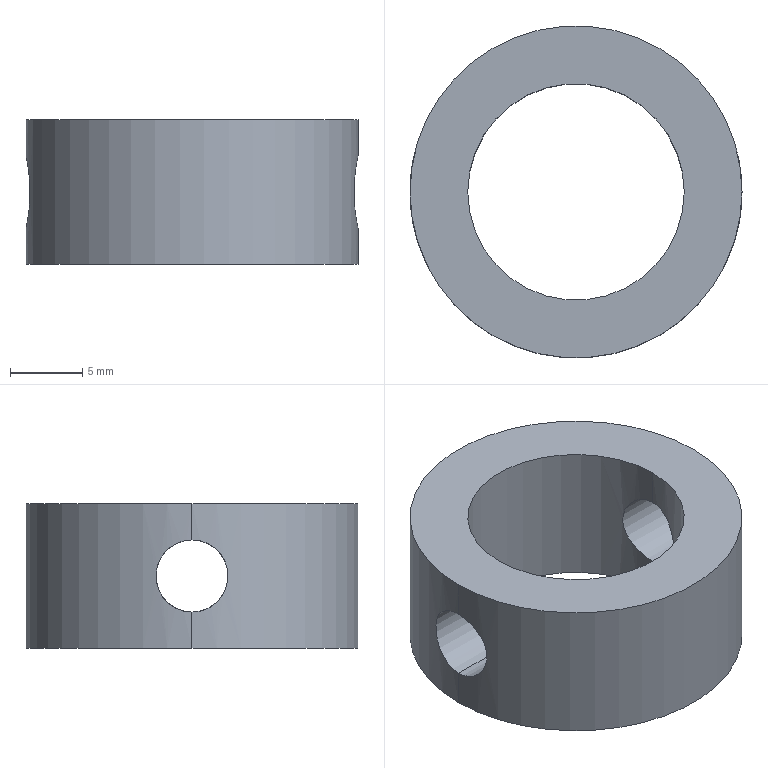Part | STEP file | X77b-01013 | 1 solid | 10 faces | box 23 x 23 x 10 mm | volume 2229 mm3 | cylinder 8 | plane 2 | commonest cylinder face diameters 5 x4 15 x2 23 x2
STEP:
#1=CARTESIAN_POINT('',(-11.5,0.,7.5));
#2=VERTEX_POINT('',#1);
#3=CARTESIAN_POINT('',(-11.5,0.,2.5));
#4=VERTEX_POINT('',#3);
#5=CARTESIAN_POINT('',(-11.5,0.,7.5));
#6=CARTESIAN_POINT('',(-11.5,-0.3268,7.5));
#7=CARTESIAN_POINT('',(-11.485,-0.6567,7.434));
#8=CARTESIAN_POINT('',(-11.447,-1.108,7.247));
#9=CARTESIAN_POINT('',(-11.432,-1.254,7.169));
#10=CARTESIAN_POINT('',(-11.399,-1.526,6.987));
#11=CARTESIAN_POINT('',(-11.381,-1.652,6.884));
#12=CARTESIAN_POINT('',(-11.346,-1.882,6.654));
#13=CARTESIAN_POINT('',(-11.327,-1.987,6.525));
#14=CARTESIAN_POINT('',(-11.294,-2.168,6.255));
#15=CARTESIAN_POINT('',(-11.279,-2.245,6.112));
#16=CARTESIAN_POINT('',(-11.24,-2.435,5.656));
#17=CARTESIAN_POINT('',(-11.225,-2.5,5.331));
#18=CARTESIAN_POINT('',(-11.225,-2.5,4.836));
#19=CARTESIAN_POINT('',(-11.229,-2.484,4.673));
#20=CARTESIAN_POINT('',(-11.242,-2.42,4.353));
#21=CARTESIAN_POINT('',(-11.253,-2.372,4.193));
#22=CARTESIAN_POINT('',(-11.279,-2.247,3.892));
#23=CARTESIAN_POINT('',(-11.294,-2.17,3.748));
#24=CARTESIAN_POINT('',(-11.327,-1.988,3.476));
#25=CARTESIAN_POINT('',(-11.345,-1.884,3.348));
#26=CARTESIAN_POINT('',(-11.399,-1.539,3.004));
#27=CARTESIAN_POINT('',(-11.435,-1.261,2.817));
#28=CARTESIAN_POINT('',(-11.472,-0.8104,2.629));
#29=CARTESIAN_POINT('',(-11.483,-0.6516,2.581));
#30=CARTESIAN_POINT('',(-11.496,-0.3291,2.516));
#31=CARTESIAN_POINT('',(-11.5,-0.1657,2.5));
#32=CARTESIAN_POINT('',(-11.5,0.,2.5));
#33=B_SPLINE_CURVE_WITH_KNOTS('',3,(#5,#6,#7,#8,#9,#10,#11,#12,#13,#14,#15,#16,#17,#18,#19,#20,#21,#22,#23,#24,#25,#26,#27,#28,#29,#30,#31,#32),.UNSPECIFIED.,.F.,.F.,(4,2,2,2,2,2,2,2,2,2,2,2,2,4),(0.00784,0.008819,0.009309,0.009799,0.01029,0.01078,0.01176,0.01225,0.01274,0.01323,0.01372,0.0147,0.01519,0.01568),.UNSPECIFIED.);
#34=EDGE_CURVE('',#2,#4,#33,.T.);
#35=ORIENTED_EDGE('',*,*,#34,.F.);
#36=CARTESIAN_POINT('',(-7.5,0.,7.5));
#37=VERTEX_POINT('',#36);
#38=CARTESIAN_POINT('',(-11.5,0.,7.5));
#39=DIRECTION('',(1.,0.,0.));
#40=VECTOR('',#39,1000.);
#41=LINE('',#38,#40);
#42=EDGE_CURVE('',#2,#37,#41,.T.);
#43=ORIENTED_EDGE('',*,*,#42,.T.);
#44=CARTESIAN_POINT('',(-7.5,0.,2.5));
#45=VERTEX_POINT('',#44);
#46=CARTESIAN_POINT('',(-7.5,0.,7.5));
#47=CARTESIAN_POINT('',(-7.5,-0.1665,7.5));
#48=CARTESIAN_POINT('',(-7.494,-0.3299,7.484));
#49=CARTESIAN_POINT('',(-7.473,-0.6511,7.419));
#50=CARTESIAN_POINT('',(-7.458,-0.8106,7.371));
#51=CARTESIAN_POINT('',(-7.419,-1.113,7.245));
#52=CARTESIAN_POINT('',(-7.395,-1.256,7.168));
#53=CARTESIAN_POINT('',(-7.344,-1.527,6.986));
#54=CARTESIAN_POINT('',(-7.316,-1.654,6.881));
#55=CARTESIAN_POINT('',(-7.233,-1.997,6.538));
#56=CARTESIAN_POINT('',(-7.176,-2.183,6.261));
#57=CARTESIAN_POINT('',(-7.116,-2.37,5.811));
#58=CARTESIAN_POINT('',(-7.099,-2.419,5.652));
#59=CARTESIAN_POINT('',(-7.077,-2.484,5.329));
#60=CARTESIAN_POINT('',(-7.071,-2.5,5.166));
#61=CARTESIAN_POINT('',(-7.071,-2.5,4.837));
#62=CARTESIAN_POINT('',(-7.077,-2.484,4.67));
#63=CARTESIAN_POINT('',(-7.099,-2.419,4.348));
#64=CARTESIAN_POINT('',(-7.116,-2.371,4.192));
#65=CARTESIAN_POINT('',(-7.156,-2.245,3.887));
#66=CARTESIAN_POINT('',(-7.181,-2.167,3.743));
#67=CARTESIAN_POINT('',(-7.233,-1.987,3.474));
#68=CARTESIAN_POINT('',(-7.261,-1.882,3.347));
#69=CARTESIAN_POINT('',(-7.317,-1.652,3.117));
#70=CARTESIAN_POINT('',(-7.344,-1.527,3.014));
#71=CARTESIAN_POINT('',(-7.395,-1.257,2.833));
#72=CARTESIAN_POINT('',(-7.419,-1.111,2.754));
#73=CARTESIAN_POINT('',(-7.458,-0.8095,2.629));
#74=CARTESIAN_POINT('',(-7.473,-0.6534,2.581));
#75=CARTESIAN_POINT('',(-7.495,-0.3297,2.516));
#76=CARTESIAN_POINT('',(-7.5,-0.164,2.5));
#77=CARTESIAN_POINT('',(-7.5,0.,2.5));
#78=B_SPLINE_CURVE_WITH_KNOTS('',3,(#46,#47,#48,#49,#50,#51,#52,#53,#54,#55,#56,#57,#58,#59,#60,#61,#62,#63,#64,#65,#66,#67,#68,#69,#70,#71,#72,#73,#74,#75,#76,#77),.UNSPECIFIED.,.F.,.F.,(4,2,2,2,2,2,2,2,2,2,2,2,2,2,2,4),(0.,0.0004921,0.0009841,0.001476,0.001968,0.002952,0.003444,0.003936,0.004429,0.004921,0.005413,0.005905,0.006397,0.006889,0.007381,0.007873),.UNSPECIFIED.);
#79=EDGE_CURVE('',#37,#45,#78,.T.);
#80=ORIENTED_EDGE('',*,*,#79,.T.);
#81=CARTESIAN_POINT('',(-11.5,0.,2.5));
#82=DIRECTION('',(1.,0.,0.));
#83=VECTOR('',#82,1000.);
#84=LINE('',#81,#83);
#85=EDGE_CURVE('',#4,#45,#84,.T.);
#86=ORIENTED_EDGE('',*,*,#85,.F.);
#87=EDGE_LOOP('',(#35,#43,#80,#86));
#88=FACE_OUTER_BOUND('',#87,.T.);
#89=CARTESIAN_POINT('',(-11.5,0.,5.));
#90=DIRECTION('',(1.,0.,0.));
#91=DIRECTION('',(0.,0.,-1.));
#92=AXIS2_PLACEMENT_3D('',#89,#90,#91);
#93=CYLINDRICAL_SURFACE('',#92,2.5);
#94=ADVANCED_FACE('',(#88),#93,.F.);
#95=CARTESIAN_POINT('',(7.5,0.,2.5));
#96=VERTEX_POINT('',#95);
#97=CARTESIAN_POINT('',(7.5,0.,7.5));
#98=VERTEX_POINT('',#97);
#99=CARTESIAN_POINT('',(7.5,0.,2.5));
#100=CARTESIAN_POINT('',(7.5,-0.1665,2.5));
#101=CARTESIAN_POINT('',(7.494,-0.3299,2.516));
#102=CARTESIAN_POINT('',(7.473,-0.6511,2.581));
#103=CARTESIAN_POINT('',(7.458,-0.8106,2.629));
#104=CARTESIAN_POINT('',(7.419,-1.113,2.755));
#105=CARTESIAN_POINT('',(7.395,-1.256,2.832));
#106=CARTESIAN_POINT('',(7.344,-1.527,3.014));
#107=CARTESIAN_POINT('',(7.316,-1.654,3.119));
#108=CARTESIAN_POINT('',(7.233,-1.997,3.462));
#109=CARTESIAN_POINT('',(7.176,-2.183,3.739));
#110=CARTESIAN_POINT('',(7.116,-2.37,4.189));
#111=CARTESIAN_POINT('',(7.099,-2.419,4.348));
#112=CARTESIAN_POINT('',(7.077,-2.484,4.671));
#113=CARTESIAN_POINT('',(7.071,-2.5,4.834));
#114=CARTESIAN_POINT('',(7.071,-2.5,5.163));
#115=CARTESIAN_POINT('',(7.077,-2.484,5.33));
#116=CARTESIAN_POINT('',(7.099,-2.419,5.652));
#117=CARTESIAN_POINT('',(7.116,-2.371,5.808));
#118=CARTESIAN_POINT('',(7.156,-2.245,6.113));
#119=CARTESIAN_POINT('',(7.181,-2.167,6.257));
#120=CARTESIAN_POINT('',(7.233,-1.987,6.526));
#121=CARTESIAN_POINT('',(7.261,-1.882,6.653));
#122=CARTESIAN_POINT('',(7.317,-1.652,6.883));
#123=CARTESIAN_POINT('',(7.344,-1.527,6.986));
#124=CARTESIAN_POINT('',(7.395,-1.257,7.167));
#125=CARTESIAN_POINT('',(7.419,-1.111,7.246));
#126=CARTESIAN_POINT('',(7.458,-0.8095,7.371));
#127=CARTESIAN_POINT('',(7.473,-0.6534,7.419));
#128=CARTESIAN_POINT('',(7.495,-0.3297,7.484));
#129=CARTESIAN_POINT('',(7.5,-0.164,7.5));
#130=CARTESIAN_POINT('',(7.5,0.,7.5));
#131=B_SPLINE_CURVE_WITH_KNOTS('',3,(#99,#100,#101,#102,#103,#104,#105,#106,#107,#108,#109,#110,#111,#112,#113,#114,#115,#116,#117,#118,#119,#120,#121,#122,#123,#124,#125,#126,#127,#128,#129,#130),.UNSPECIFIED.,.F.,.F.,(4,2,2,2,2,2,2,2,2,2,2,2,2,2,2,4),(0.,0.0004921,0.0009841,0.001476,0.001968,0.002952,0.003444,0.003936,0.004429,0.004921,0.005413,0.005905,0.006397,0.006889,0.007381,0.007873),.UNSPECIFIED.);
#132=EDGE_CURVE('',#96,#98,#131,.T.);
#133=ORIENTED_EDGE('',*,*,#132,.T.);
#134=CARTESIAN_POINT('',(11.5,0.,7.5));
#135=VERTEX_POINT('',#134);
#136=CARTESIAN_POINT('',(-11.5,0.,7.5));
#137=DIRECTION('',(1.,0.,0.));
#138=VECTOR('',#137,1000.);
#139=LINE('',#136,#138);
#140=EDGE_CURVE('',#98,#135,#139,.T.);
#141=ORIENTED_EDGE('',*,*,#140,.T.);
#142=CARTESIAN_POINT('',(11.5,0.,2.5));
#143=VERTEX_POINT('',#142);
#144=CARTESIAN_POINT('',(11.5,0.,2.5));
#145=CARTESIAN_POINT('',(11.5,-0.1657,2.5));
#146=CARTESIAN_POINT('',(11.496,-0.3286,2.516));
#147=CARTESIAN_POINT('',(11.483,-0.6488,2.58));
#148=CARTESIAN_POINT('',(11.473,-0.8079,2.628));
#149=CARTESIAN_POINT('',(11.447,-1.11,2.754));
#150=CARTESIAN_POINT('',(11.432,-1.254,2.831));
#151=CARTESIAN_POINT('',(11.399,-1.525,3.012));
#152=CARTESIAN_POINT('',(11.381,-1.653,3.118));
#153=CARTESIAN_POINT('',(11.327,-1.998,3.463));
#154=CARTESIAN_POINT('',(11.291,-2.184,3.741));
#155=CARTESIAN_POINT('',(11.253,-2.371,4.192));
#156=CARTESIAN_POINT('',(11.243,-2.42,4.35));
#157=CARTESIAN_POINT('',(11.229,-2.484,4.673));
#158=CARTESIAN_POINT('',(11.225,-2.5,4.835));
#159=CARTESIAN_POINT('',(11.225,-2.5,5.163));
#160=CARTESIAN_POINT('',(11.229,-2.484,5.329));
#161=CARTESIAN_POINT('',(11.243,-2.42,5.65));
#162=CARTESIAN_POINT('',(11.253,-2.372,5.806));
#163=CARTESIAN_POINT('',(11.279,-2.246,6.109));
#164=CARTESIAN_POINT('',(11.294,-2.168,6.255));
#165=CARTESIAN_POINT('',(11.327,-1.988,6.525));
#166=CARTESIAN_POINT('',(11.345,-1.884,6.652));
#167=CARTESIAN_POINT('',(11.381,-1.651,6.884));
#168=CARTESIAN_POINT('',(11.399,-1.526,6.987));
#169=CARTESIAN_POINT('',(11.432,-1.255,7.168));
#170=CARTESIAN_POINT('',(11.447,-1.109,7.247));
#171=CARTESIAN_POINT('',(11.473,-0.8068,7.372));
#172=CARTESIAN_POINT('',(11.483,-0.651,7.419));
#173=CARTESIAN_POINT('',(11.496,-0.3294,7.484));
#174=CARTESIAN_POINT('',(11.5,-0.1634,7.5));
#175=CARTESIAN_POINT('',(11.5,0.,7.5));
#176=B_SPLINE_CURVE_WITH_KNOTS('',3,(#144,#145,#146,#147,#148,#149,#150,#151,#152,#153,#154,#155,#156,#157,#158,#159,#160,#161,#162,#163,#164,#165,#166,#167,#168,#169,#170,#171,#172,#173,#174,#175),.UNSPECIFIED.,.F.,.F.,(4,2,2,2,2,2,2,2,2,2,2,2,2,2,2,4),(0.,0.00049,0.0009799,0.00147,0.00196,0.00294,0.00343,0.00392,0.00441,0.0049,0.00539,0.00588,0.00637,0.00686,0.00735,0.00784),.UNSPECIFIED.);
#177=EDGE_CURVE('',#143,#135,#176,.T.);
#178=ORIENTED_EDGE('',*,*,#177,.F.);
#179=CARTESIAN_POINT('',(-11.5,0.,2.5));
#180=DIRECTION('',(1.,0.,0.));
#181=VECTOR('',#180,1000.);
#182=LINE('',#179,#181);
#183=EDGE_CURVE('',#96,#143,#182,.T.);
#184=ORIENTED_EDGE('',*,*,#183,.F.);
#185=EDGE_LOOP('',(#133,#141,#178,#184));
#186=FACE_OUTER_BOUND('',#185,.T.);
#187=CARTESIAN_POINT('',(-11.5,0.,5.));
#188=DIRECTION('',(1.,0.,0.));
#189=DIRECTION('',(0.,0.,-1.));
#190=AXIS2_PLACEMENT_3D('',#187,#188,#189);
#191=CYLINDRICAL_SURFACE('',#190,2.5);
#192=ADVANCED_FACE('',(#186),#191,.F.);
#193=CARTESIAN_POINT('',(-7.5,0.,10.));
#194=VERTEX_POINT('',#193);
#195=CARTESIAN_POINT('',(7.5,0.,10.));
#196=VERTEX_POINT('',#195);
#197=CARTESIAN_POINT('',(0.,0.,10.));
#198=DIRECTION('',(0.,0.,1.));
#199=DIRECTION('',(1.,0.,0.));
#200=AXIS2_PLACEMENT_3D('',#197,#198,#199);
#201=CIRCLE('',#200,7.5);
#202=EDGE_CURVE('',#194,#196,#201,.T.);
#203=ORIENTED_EDGE('',*,*,#202,.T.);
#204=CARTESIAN_POINT('',(7.5,0.,10.));
#205=DIRECTION('',(0.,0.,-1.));
#206=VECTOR('',#205,1000.);
#207=LINE('',#204,#206);
#208=EDGE_CURVE('',#196,#98,#207,.T.);
#209=ORIENTED_EDGE('',*,*,#208,.T.);
#210=ORIENTED_EDGE('',*,*,#132,.F.);
#211=CARTESIAN_POINT('',(7.5,0.,0.));
#212=VERTEX_POINT('',#211);
#213=CARTESIAN_POINT('',(7.5,0.,10.));
#214=DIRECTION('',(0.,0.,-1.));
#215=VECTOR('',#214,1000.);
#216=LINE('',#213,#215);
#217=EDGE_CURVE('',#96,#212,#216,.T.);
#218=ORIENTED_EDGE('',*,*,#217,.T.);
#219=CARTESIAN_POINT('',(-7.5,0.,0.));
#220=VERTEX_POINT('',#219);
#221=CARTESIAN_POINT('',(0.,0.,0.));
#222=DIRECTION('',(0.,0.,1.));
#223=DIRECTION('',(1.,0.,0.));
#224=AXIS2_PLACEMENT_3D('',#221,#222,#223);
#225=CIRCLE('',#224,7.5);
#226=EDGE_CURVE('',#220,#212,#225,.T.);
#227=ORIENTED_EDGE('',*,*,#226,.F.);
#228=CARTESIAN_POINT('',(-7.5,0.,10.));
#229=DIRECTION('',(0.,0.,-1.));
#230=VECTOR('',#229,1000.);
#231=LINE('',#228,#230);
#232=EDGE_CURVE('',#45,#220,#231,.T.);
#233=ORIENTED_EDGE('',*,*,#232,.F.);
#234=ORIENTED_EDGE('',*,*,#79,.F.);
#235=CARTESIAN_POINT('',(-7.5,0.,10.));
#236=DIRECTION('',(0.,0.,-1.));
#237=VECTOR('',#236,1000.);
#238=LINE('',#235,#237);
#239=EDGE_CURVE('',#194,#37,#238,.T.);
#240=ORIENTED_EDGE('',*,*,#239,.F.);
#241=EDGE_LOOP('',(#203,#209,#210,#218,#227,#233,#234,#240));
#242=FACE_OUTER_BOUND('',#241,.T.);
#243=CARTESIAN_POINT('',(0.,0.,10.));
#244=DIRECTION('',(0.,0.,-1.));
#245=DIRECTION('',(-1.,0.,0.));
#246=AXIS2_PLACEMENT_3D('',#243,#244,#245);
#247=CYLINDRICAL_SURFACE('',#246,7.5);
#248=ADVANCED_FACE('',(#242),#247,.F.);
#249=CARTESIAN_POINT('',(11.5,0.,10.));
#250=VERTEX_POINT('',#249);
#251=CARTESIAN_POINT('',(-11.5,0.,10.));
#252=VERTEX_POINT('',#251);
#253=CARTESIAN_POINT('',(0.,0.,10.));
#254=DIRECTION('',(0.,0.,1.));
#255=DIRECTION('',(1.,0.,0.));
#256=AXIS2_PLACEMENT_3D('',#253,#254,#255);
#257=CIRCLE('',#256,11.5);
#258=EDGE_CURVE('',#250,#252,#257,.T.);
#259=ORIENTED_EDGE('',*,*,#258,.F.);
#260=CARTESIAN_POINT('',(11.5,0.,10.));
#261=DIRECTION('',(0.,0.,-1.));
#262=VECTOR('',#261,1000.);
#263=LINE('',#260,#262);
#264=EDGE_CURVE('',#250,#135,#263,.T.);
#265=ORIENTED_EDGE('',*,*,#264,.T.);
#266=CARTESIAN_POINT('',(11.5,0.,7.5));
#267=CARTESIAN_POINT('',(11.5,0.3268,7.5));
#268=CARTESIAN_POINT('',(11.485,0.6567,7.434));
#269=CARTESIAN_POINT('',(11.447,1.108,7.247));
#270=CARTESIAN_POINT('',(11.432,1.254,7.169));
#271=CARTESIAN_POINT('',(11.399,1.526,6.987));
#272=CARTESIAN_POINT('',(11.381,1.652,6.884));
#273=CARTESIAN_POINT('',(11.346,1.882,6.654));
#274=CARTESIAN_POINT('',(11.327,1.987,6.525));
#275=CARTESIAN_POINT('',(11.294,2.168,6.255));
#276=CARTESIAN_POINT('',(11.279,2.245,6.112));
#277=CARTESIAN_POINT('',(11.24,2.435,5.656));
#278=CARTESIAN_POINT('',(11.225,2.5,5.331));
#279=CARTESIAN_POINT('',(11.225,2.5,4.836));
#280=CARTESIAN_POINT('',(11.229,2.484,4.673));
#281=CARTESIAN_POINT('',(11.242,2.42,4.353));
#282=CARTESIAN_POINT('',(11.253,2.372,4.193));
#283=CARTESIAN_POINT('',(11.279,2.247,3.892));
#284=CARTESIAN_POINT('',(11.294,2.17,3.748));
#285=CARTESIAN_POINT('',(11.327,1.988,3.476));
#286=CARTESIAN_POINT('',(11.345,1.884,3.348));
#287=CARTESIAN_POINT('',(11.399,1.539,3.004));
#288=CARTESIAN_POINT('',(11.435,1.261,2.817));
#289=CARTESIAN_POINT('',(11.472,0.8104,2.629));
#290=CARTESIAN_POINT('',(11.483,0.6516,2.581));
#291=CARTESIAN_POINT('',(11.496,0.3291,2.516));
#292=CARTESIAN_POINT('',(11.5,0.1657,2.5));
#293=CARTESIAN_POINT('',(11.5,0.,2.5));
#294=B_SPLINE_CURVE_WITH_KNOTS('',3,(#266,#267,#268,#269,#270,#271,#272,#273,#274,#275,#276,#277,#278,#279,#280,#281,#282,#283,#284,#285,#286,#287,#288,#289,#290,#291,#292,#293),.UNSPECIFIED.,.F.,.F.,(4,2,2,2,2,2,2,2,2,2,2,2,2,4),(0.00784,0.008819,0.009309,0.009799,0.01029,0.01078,0.01176,0.01225,0.01274,0.01323,0.01372,0.0147,0.01519,0.01568),.UNSPECIFIED.);
#295=EDGE_CURVE('',#135,#143,#294,.T.);
#296=ORIENTED_EDGE('',*,*,#295,.T.);
#297=CARTESIAN_POINT('',(11.5,0.,0.));
#298=VERTEX_POINT('',#297);
#299=CARTESIAN_POINT('',(11.5,0.,10.));
#300=DIRECTION('',(0.,0.,-1.));
#301=VECTOR('',#300,1000.);
#302=LINE('',#299,#301);
#303=EDGE_CURVE('',#143,#298,#302,.T.);
#304=ORIENTED_EDGE('',*,*,#303,.T.);
#305=CARTESIAN_POINT('',(-11.5,0.,0.));
#306=VERTEX_POINT('',#305);
#307=CARTESIAN_POINT('',(0.,0.,0.));
#308=DIRECTION('',(0.,0.,1.));
#309=DIRECTION('',(1.,0.,0.));
#310=AXIS2_PLACEMENT_3D('',#307,#308,#309);
#311=CIRCLE('',#310,11.5);
#312=EDGE_CURVE('',#298,#306,#311,.T.);
#313=ORIENTED_EDGE('',*,*,#312,.T.);
#314=CARTESIAN_POINT('',(-11.5,0.,10.));
#315=DIRECTION('',(0.,0.,-1.));
#316=VECTOR('',#315,1000.);
#317=LINE('',#314,#316);
#318=EDGE_CURVE('',#4,#306,#317,.T.);
#319=ORIENTED_EDGE('',*,*,#318,.F.);
#320=CARTESIAN_POINT('',(-11.5,0.,2.5));
#321=CARTESIAN_POINT('',(-11.5,0.1657,2.5));
#322=CARTESIAN_POINT('',(-11.496,0.3286,2.516));
#323=CARTESIAN_POINT('',(-11.483,0.6488,2.58));
#324=CARTESIAN_POINT('',(-11.473,0.8079,2.628));
#325=CARTESIAN_POINT('',(-11.447,1.11,2.754));
#326=CARTESIAN_POINT('',(-11.432,1.254,2.831));
#327=CARTESIAN_POINT('',(-11.399,1.525,3.012));
#328=CARTESIAN_POINT('',(-11.381,1.653,3.118));
#329=CARTESIAN_POINT('',(-11.327,1.998,3.463));
#330=CARTESIAN_POINT('',(-11.291,2.184,3.741));
#331=CARTESIAN_POINT('',(-11.253,2.371,4.192));
#332=CARTESIAN_POINT('',(-11.243,2.42,4.35));
#333=CARTESIAN_POINT('',(-11.229,2.484,4.673));
#334=CARTESIAN_POINT('',(-11.225,2.5,4.835));
#335=CARTESIAN_POINT('',(-11.225,2.5,5.163));
#336=CARTESIAN_POINT('',(-11.229,2.484,5.329));
#337=CARTESIAN_POINT('',(-11.243,2.42,5.65));
#338=CARTESIAN_POINT('',(-11.253,2.372,5.806));
#339=CARTESIAN_POINT('',(-11.279,2.246,6.109));
#340=CARTESIAN_POINT('',(-11.294,2.168,6.255));
#341=CARTESIAN_POINT('',(-11.327,1.988,6.525));
#342=CARTESIAN_POINT('',(-11.345,1.884,6.652));
#343=CARTESIAN_POINT('',(-11.381,1.651,6.884));
#344=CARTESIAN_POINT('',(-11.399,1.526,6.987));
#345=CARTESIAN_POINT('',(-11.432,1.255,7.168));
#346=CARTESIAN_POINT('',(-11.447,1.109,7.247));
#347=CARTESIAN_POINT('',(-11.473,0.8068,7.372));
#348=CARTESIAN_POINT('',(-11.483,0.651,7.419));
#349=CARTESIAN_POINT('',(-11.496,0.3294,7.484));
#350=CARTESIAN_POINT('',(-11.5,0.1634,7.5));
#351=CARTESIAN_POINT('',(-11.5,0.,7.5));
#352=B_SPLINE_CURVE_WITH_KNOTS('',3,(#320,#321,#322,#323,#324,#325,#326,#327,#328,#329,#330,#331,#332,#333,#334,#335,#336,#337,#338,#339,#340,#341,#342,#343,#344,#345,#346,#347,#348,#349,#350,#351),.UNSPECIFIED.,.F.,.F.,(4,2,2,2,2,2,2,2,2,2,2,2,2,2,2,4),(0.,0.00049,0.0009799,0.00147,0.00196,0.00294,0.00343,0.00392,0.00441,0.0049,0.00539,0.00588,0.00637,0.00686,0.00735,0.00784),.UNSPECIFIED.);
#353=EDGE_CURVE('',#4,#2,#352,.T.);
#354=ORIENTED_EDGE('',*,*,#353,.T.);
#355=CARTESIAN_POINT('',(-11.5,0.,10.));
#356=DIRECTION('',(0.,0.,-1.));
#357=VECTOR('',#356,1000.);
#358=LINE('',#355,#357);
#359=EDGE_CURVE('',#252,#2,#358,.T.);
#360=ORIENTED_EDGE('',*,*,#359,.F.);
#361=EDGE_LOOP('',(#259,#265,#296,#304,#313,#319,#354,#360));
#362=FACE_OUTER_BOUND('',#361,.T.);
#363=CARTESIAN_POINT('',(0.,0.,10.));
#364=DIRECTION('',(0.,0.,-1.));
#365=DIRECTION('',(-1.,0.,0.));
#366=AXIS2_PLACEMENT_3D('',#363,#364,#365);
#367=CYLINDRICAL_SURFACE('',#366,11.5);
#368=ADVANCED_FACE('',(#362),#367,.T.);
#369=CARTESIAN_POINT('',(0.,0.,10.));
#370=DIRECTION('',(0.,0.,1.));
#371=DIRECTION('',(1.,0.,0.));
#372=AXIS2_PLACEMENT_3D('',#369,#370,#371);
#373=CIRCLE('',#372,11.5);
#374=EDGE_CURVE('',#252,#250,#373,.T.);
#375=ORIENTED_EDGE('',*,*,#374,.T.);
#376=ORIENTED_EDGE('',*,*,#258,.T.);
#377=EDGE_LOOP('',(#375,#376));
#378=FACE_OUTER_BOUND('',#377,.T.);
#379=ORIENTED_EDGE('',*,*,#202,.F.);
#380=CARTESIAN_POINT('',(0.,0.,10.));
#381=DIRECTION('',(0.,0.,1.));
#382=DIRECTION('',(1.,0.,0.));
#383=AXIS2_PLACEMENT_3D('',#380,#381,#382);
#384=CIRCLE('',#383,7.5);
#385=EDGE_CURVE('',#196,#194,#384,.T.);
#386=ORIENTED_EDGE('',*,*,#385,.F.);
#387=EDGE_LOOP('',(#379,#386));
#388=FACE_BOUND('',#387,.T.);
#389=CARTESIAN_POINT('',(0.,0.,10.));
#390=DIRECTION('',(0.,0.,1.));
#391=DIRECTION('',(1.,0.,0.));
#392=AXIS2_PLACEMENT_3D('',#389,#390,#391);
#393=PLANE('',#392);
#394=ADVANCED_FACE('',(#378,#388),#393,.T.);
#395=CARTESIAN_POINT('',(0.,0.,0.));
#396=DIRECTION('',(0.,0.,1.));
#397=DIRECTION('',(1.,0.,0.));
#398=AXIS2_PLACEMENT_3D('',#395,#396,#397);
#399=CIRCLE('',#398,11.5);
#400=EDGE_CURVE('',#306,#298,#399,.T.);
#401=ORIENTED_EDGE('',*,*,#400,.F.);
#402=ORIENTED_EDGE('',*,*,#312,.F.);
#403=EDGE_LOOP('',(#401,#402));
#404=FACE_OUTER_BOUND('',#403,.T.);
#405=ORIENTED_EDGE('',*,*,#226,.T.);
#406=CARTESIAN_POINT('',(0.,0.,0.));
#407=DIRECTION('',(0.,0.,1.));
#408=DIRECTION('',(1.,0.,0.));
#409=AXIS2_PLACEMENT_3D('',#406,#407,#408);
#410=CIRCLE('',#409,7.5);
#411=EDGE_CURVE('',#212,#220,#410,.T.);
#412=ORIENTED_EDGE('',*,*,#411,.T.);
#413=EDGE_LOOP('',(#405,#412));
#414=FACE_BOUND('',#413,.T.);
#415=CARTESIAN_POINT('',(0.,0.,0.));
#416=DIRECTION('',(0.,0.,1.));
#417=DIRECTION('',(1.,0.,0.));
#418=AXIS2_PLACEMENT_3D('',#415,#416,#417);
#419=PLANE('',#418);
#420=ADVANCED_FACE('',(#404,#414),#419,.F.);
#421=ORIENTED_EDGE('',*,*,#264,.F.);
#422=ORIENTED_EDGE('',*,*,#374,.F.);
#423=ORIENTED_EDGE('',*,*,#359,.T.);
#424=ORIENTED_EDGE('',*,*,#34,.T.);
#425=ORIENTED_EDGE('',*,*,#318,.T.);
#426=ORIENTED_EDGE('',*,*,#400,.T.);
#427=ORIENTED_EDGE('',*,*,#303,.F.);
#428=ORIENTED_EDGE('',*,*,#177,.T.);
#429=EDGE_LOOP('',(#421,#422,#423,#424,#425,#426,#427,#428));
#430=FACE_OUTER_BOUND('',#429,.T.);
#431=CARTESIAN_POINT('',(0.,0.,10.));
#432=DIRECTION('',(0.,0.,-1.));
#433=DIRECTION('',(-1.,0.,0.));
#434=AXIS2_PLACEMENT_3D('',#431,#432,#433);
#435=CYLINDRICAL_SURFACE('',#434,11.5);
#436=ADVANCED_FACE('',(#430),#435,.T.);
#437=ORIENTED_EDGE('',*,*,#208,.F.);
#438=ORIENTED_EDGE('',*,*,#385,.T.);
#439=ORIENTED_EDGE('',*,*,#239,.T.);
#440=CARTESIAN_POINT('',(-7.5,0.,2.5));
#441=CARTESIAN_POINT('',(-7.5,0.1639,2.5));
#442=CARTESIAN_POINT('',(-7.495,0.329,2.516));
#443=CARTESIAN_POINT('',(-7.473,0.6534,2.581));
#444=CARTESIAN_POINT('',(-7.458,0.8097,2.629));
#445=CARTESIAN_POINT('',(-7.419,1.111,2.755));
#446=CARTESIAN_POINT('',(-7.395,1.258,2.833));
#447=CARTESIAN_POINT('',(-7.344,1.528,3.014));
#448=CARTESIAN_POINT('',(-7.317,1.653,3.117));
#449=CARTESIAN_POINT('',(-7.233,1.999,3.463));
#450=CARTESIAN_POINT('',(-7.177,2.182,3.736));
#451=CARTESIAN_POINT('',(-7.116,2.371,4.192));
#452=CARTESIAN_POINT('',(-7.099,2.419,4.348));
#453=CARTESIAN_POINT('',(-7.077,2.483,4.669));
#454=CARTESIAN_POINT('',(-7.071,2.5,4.836));
#455=CARTESIAN_POINT('',(-7.071,2.5,5.165));
#456=CARTESIAN_POINT('',(-7.077,2.484,5.328));
#457=CARTESIAN_POINT('',(-7.099,2.419,5.651));
#458=CARTESIAN_POINT('',(-7.116,2.371,5.81));
#459=CARTESIAN_POINT('',(-7.177,2.183,6.262));
#460=CARTESIAN_POINT('',(-7.233,1.997,6.538));
#461=CARTESIAN_POINT('',(-7.316,1.654,6.882));
#462=CARTESIAN_POINT('',(-7.344,1.526,6.987));
#463=CARTESIAN_POINT('',(-7.395,1.256,7.168));
#464=CARTESIAN_POINT('',(-7.419,1.113,7.245));
#465=CARTESIAN_POINT('',(-7.458,0.8105,7.371));
#466=CARTESIAN_POINT('',(-7.473,0.651,7.419));
#467=CARTESIAN_POINT('',(-7.494,0.3299,7.484));
#468=CARTESIAN_POINT('',(-7.5,0.1664,7.5));
#469=CARTESIAN_POINT('',(-7.5,0.,7.5));
#470=B_SPLINE_CURVE_WITH_KNOTS('',3,(#440,#441,#442,#443,#444,#445,#446,#447,#448,#449,#450,#451,#452,#453,#454,#455,#456,#457,#458,#459,#460,#461,#462,#463,#464,#465,#466,#467,#468,#469),.UNSPECIFIED.,.F.,.F.,(4,2,2,2,2,2,2,2,2,2,2,2,2,2,4),(0.007873,0.008365,0.008857,0.009349,0.009841,0.01082,0.01132,0.01181,0.0123,0.01279,0.01378,0.01427,0.01476,0.01525,0.01574),.UNSPECIFIED.);
#471=EDGE_CURVE('',#45,#37,#470,.T.);
#472=ORIENTED_EDGE('',*,*,#471,.F.);
#473=ORIENTED_EDGE('',*,*,#232,.T.);
#474=ORIENTED_EDGE('',*,*,#411,.F.);
#475=ORIENTED_EDGE('',*,*,#217,.F.);
#476=CARTESIAN_POINT('',(7.5,0.,7.5));
#477=CARTESIAN_POINT('',(7.5,0.1639,7.5));
#478=CARTESIAN_POINT('',(7.495,0.329,7.484));
#479=CARTESIAN_POINT('',(7.473,0.6534,7.419));
#480=CARTESIAN_POINT('',(7.458,0.8097,7.371));
#481=CARTESIAN_POINT('',(7.419,1.111,7.245));
#482=CARTESIAN_POINT('',(7.395,1.258,7.167));
#483=CARTESIAN_POINT('',(7.344,1.528,6.986));
#484=CARTESIAN_POINT('',(7.317,1.653,6.883));
#485=CARTESIAN_POINT('',(7.233,1.999,6.537));
#486=CARTESIAN_POINT('',(7.177,2.182,6.264));
#487=CARTESIAN_POINT('',(7.116,2.371,5.808));
#488=CARTESIAN_POINT('',(7.099,2.419,5.652));
#489=CARTESIAN_POINT('',(7.077,2.483,5.331));
#490=CARTESIAN_POINT('',(7.071,2.5,5.164));
#491=CARTESIAN_POINT('',(7.071,2.5,4.835));
#492=CARTESIAN_POINT('',(7.077,2.484,4.672));
#493=CARTESIAN_POINT('',(7.099,2.419,4.349));
#494=CARTESIAN_POINT('',(7.116,2.371,4.19));
#495=CARTESIAN_POINT('',(7.177,2.183,3.738));
#496=CARTESIAN_POINT('',(7.233,1.997,3.462));
#497=CARTESIAN_POINT('',(7.316,1.654,3.118));
#498=CARTESIAN_POINT('',(7.344,1.526,3.013));
#499=CARTESIAN_POINT('',(7.395,1.256,2.832));
#500=CARTESIAN_POINT('',(7.419,1.113,2.755));
#501=CARTESIAN_POINT('',(7.458,0.8105,2.629));
#502=CARTESIAN_POINT('',(7.473,0.651,2.581));
#503=CARTESIAN_POINT('',(7.494,0.3299,2.516));
#504=CARTESIAN_POINT('',(7.5,0.1664,2.5));
#505=CARTESIAN_POINT('',(7.5,0.,2.5));
#506=B_SPLINE_CURVE_WITH_KNOTS('',3,(#476,#477,#478,#479,#480,#481,#482,#483,#484,#485,#486,#487,#488,#489,#490,#491,#492,#493,#494,#495,#496,#497,#498,#499,#500,#501,#502,#503,#504,#505),.UNSPECIFIED.,.F.,.F.,(4,2,2,2,2,2,2,2,2,2,2,2,2,2,4),(0.007873,0.008365,0.008857,0.009349,0.009841,0.01082,0.01132,0.01181,0.0123,0.01279,0.01378,0.01427,0.01476,0.01525,0.01574),.UNSPECIFIED.);
#507=EDGE_CURVE('',#98,#96,#506,.T.);
#508=ORIENTED_EDGE('',*,*,#507,.F.);
#509=EDGE_LOOP('',(#437,#438,#439,#472,#473,#474,#475,#508));
#510=FACE_OUTER_BOUND('',#509,.T.);
#511=CARTESIAN_POINT('',(0.,0.,10.));
#512=DIRECTION('',(0.,0.,-1.));
#513=DIRECTION('',(-1.,0.,0.));
#514=AXIS2_PLACEMENT_3D('',#511,#512,#513);
#515=CYLINDRICAL_SURFACE('',#514,7.5);
#516=ADVANCED_FACE('',(#510),#515,.F.);
#517=ORIENTED_EDGE('',*,*,#140,.F.);
#518=ORIENTED_EDGE('',*,*,#507,.T.);
#519=ORIENTED_EDGE('',*,*,#183,.T.);
#520=ORIENTED_EDGE('',*,*,#295,.F.);
#521=EDGE_LOOP('',(#517,#518,#519,#520));
#522=FACE_OUTER_BOUND('',#521,.T.);
#523=CARTESIAN_POINT('',(-11.5,0.,5.));
#524=DIRECTION('',(1.,0.,0.));
#525=DIRECTION('',(0.,0.,-1.));
#526=AXIS2_PLACEMENT_3D('',#523,#524,#525);
#527=CYLINDRICAL_SURFACE('',#526,2.5);
#528=ADVANCED_FACE('',(#522),#527,.F.);
#529=ORIENTED_EDGE('',*,*,#42,.F.);
#530=ORIENTED_EDGE('',*,*,#353,.F.);
#531=ORIENTED_EDGE('',*,*,#85,.T.);
#532=ORIENTED_EDGE('',*,*,#471,.T.);
#533=EDGE_LOOP('',(#529,#530,#531,#532));
#534=FACE_OUTER_BOUND('',#533,.T.);
#535=CARTESIAN_POINT('',(-11.5,0.,5.));
#536=DIRECTION('',(1.,0.,0.));
#537=DIRECTION('',(0.,0.,-1.));
#538=AXIS2_PLACEMENT_3D('',#535,#536,#537);
#539=CYLINDRICAL_SURFACE('',#538,2.5);
#540=ADVANCED_FACE('',(#534),#539,.F.);
#541=CLOSED_SHELL('',(#94,#192,#248,#368,#394,#420,#436,#516,#528,#540));
#542=MANIFOLD_SOLID_BREP('',#541);
#543=CARTESIAN_POINT('',(0.,0.,0.));
#544=DIRECTION('',(0.,0.,1.));
#545=DIRECTION('',(1.,0.,0.));
#546=AXIS2_PLACEMENT_3D('',#543,#544,#545);
#547=(LENGTH_UNIT()NAMED_UNIT(*)SI_UNIT(.MILLI.,.METRE.));
#548=UNCERTAINTY_MEASURE_WITH_UNIT(LENGTH_MEASURE(0.00001),#547,'','');
#549=(NAMED_UNIT(*)PLANE_ANGLE_UNIT()SI_UNIT($,.RADIAN.));
#550=(NAMED_UNIT(*)SI_UNIT($,.STERADIAN.)SOLID_ANGLE_UNIT());
#551=(GEOMETRIC_REPRESENTATION_CONTEXT(3)GLOBAL_UNCERTAINTY_ASSIGNED_CONTEXT((#548))GLOBAL_UNIT_ASSIGNED_CONTEXT((#547,#549,#550))REPRESENTATION_CONTEXT('',''));
#552=ADVANCED_BREP_SHAPE_REPRESENTATION('',(#542,#546),#551);